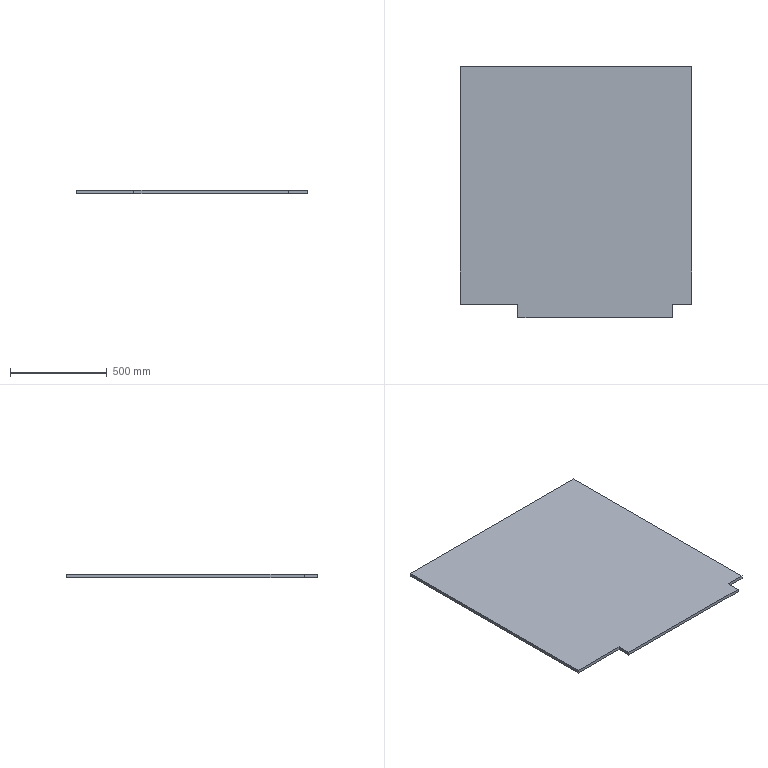Part | 1 solid | 10 faces | box 1198 x 1299 x 16 mm | volume 24453472 mm3 | plane 10
STEP:
#1=CARTESIAN_POINT('',(-599.,500.,0.));
#2=VERTEX_POINT('',#1);
#3=CARTESIAN_POINT('',(-599.,-729.,0.));
#4=VERTEX_POINT('',#3);
#5=CARTESIAN_POINT('',(-599.,500.,0.));
#6=DIRECTION('',(0.,-1.,0.));
#7=VECTOR('',#6,1000.);
#8=LINE('',#5,#7);
#9=EDGE_CURVE('',#2,#4,#8,.T.);
#10=ORIENTED_EDGE('',*,*,#9,.T.);
#11=CARTESIAN_POINT('',(-599.,-729.,16.));
#12=VERTEX_POINT('',#11);
#13=CARTESIAN_POINT('',(-599.,-729.,16.));
#14=DIRECTION('',(0.,0.,-1.));
#15=VECTOR('',#14,1000.);
#16=LINE('',#13,#15);
#17=EDGE_CURVE('',#12,#4,#16,.T.);
#18=ORIENTED_EDGE('',*,*,#17,.F.);
#19=CARTESIAN_POINT('',(-599.,500.,16.));
#20=VERTEX_POINT('',#19);
#21=CARTESIAN_POINT('',(-599.,500.,16.));
#22=DIRECTION('',(0.,-1.,0.));
#23=VECTOR('',#22,1000.);
#24=LINE('',#21,#23);
#25=EDGE_CURVE('',#20,#12,#24,.T.);
#26=ORIENTED_EDGE('',*,*,#25,.F.);
#27=CARTESIAN_POINT('',(-599.,500.,16.));
#28=DIRECTION('',(0.,0.,-1.));
#29=VECTOR('',#28,1000.);
#30=LINE('',#27,#29);
#31=EDGE_CURVE('',#20,#2,#30,.T.);
#32=ORIENTED_EDGE('',*,*,#31,.T.);
#33=EDGE_LOOP('',(#10,#18,#26,#32));
#34=FACE_OUTER_BOUND('',#33,.T.);
#35=CARTESIAN_POINT('',(-599.,500.,16.));
#36=DIRECTION('',(1.,0.,0.));
#37=DIRECTION('',(0.,1.,0.));
#38=AXIS2_PLACEMENT_3D('',#35,#36,#37);
#39=PLANE('',#38);
#40=ADVANCED_FACE('',(#34),#39,.F.);
#41=CARTESIAN_POINT('',(-300.,-729.,0.));
#42=VERTEX_POINT('',#41);
#43=CARTESIAN_POINT('',(-599.,-729.,0.));
#44=DIRECTION('',(1.,0.,0.));
#45=VECTOR('',#44,1000.);
#46=LINE('',#43,#45);
#47=EDGE_CURVE('',#4,#42,#46,.T.);
#48=ORIENTED_EDGE('',*,*,#47,.T.);
#49=CARTESIAN_POINT('',(-300.,-729.,16.));
#50=VERTEX_POINT('',#49);
#51=CARTESIAN_POINT('',(-300.,-729.,16.));
#52=DIRECTION('',(0.,0.,-1.));
#53=VECTOR('',#52,1000.);
#54=LINE('',#51,#53);
#55=EDGE_CURVE('',#50,#42,#54,.T.);
#56=ORIENTED_EDGE('',*,*,#55,.F.);
#57=CARTESIAN_POINT('',(-599.,-729.,16.));
#58=DIRECTION('',(1.,0.,0.));
#59=VECTOR('',#58,1000.);
#60=LINE('',#57,#59);
#61=EDGE_CURVE('',#12,#50,#60,.T.);
#62=ORIENTED_EDGE('',*,*,#61,.F.);
#63=ORIENTED_EDGE('',*,*,#17,.T.);
#64=EDGE_LOOP('',(#48,#56,#62,#63));
#65=FACE_OUTER_BOUND('',#64,.T.);
#66=CARTESIAN_POINT('',(-599.,-729.,16.));
#67=DIRECTION('',(0.,1.,0.));
#68=DIRECTION('',(0.,0.,1.));
#69=AXIS2_PLACEMENT_3D('',#66,#67,#68);
#70=PLANE('',#69);
#71=ADVANCED_FACE('',(#65),#70,.F.);
#72=CARTESIAN_POINT('',(-300.,-799.,0.));
#73=VERTEX_POINT('',#72);
#74=CARTESIAN_POINT('',(-300.,-729.,0.));
#75=DIRECTION('',(0.,-1.,0.));
#76=VECTOR('',#75,1000.);
#77=LINE('',#74,#76);
#78=EDGE_CURVE('',#42,#73,#77,.T.);
#79=ORIENTED_EDGE('',*,*,#78,.T.);
#80=CARTESIAN_POINT('',(-300.,-799.,16.));
#81=VERTEX_POINT('',#80);
#82=CARTESIAN_POINT('',(-300.,-799.,16.));
#83=DIRECTION('',(0.,0.,-1.));
#84=VECTOR('',#83,1000.);
#85=LINE('',#82,#84);
#86=EDGE_CURVE('',#81,#73,#85,.T.);
#87=ORIENTED_EDGE('',*,*,#86,.F.);
#88=CARTESIAN_POINT('',(-300.,-729.,16.));
#89=DIRECTION('',(0.,-1.,0.));
#90=VECTOR('',#89,1000.);
#91=LINE('',#88,#90);
#92=EDGE_CURVE('',#50,#81,#91,.T.);
#93=ORIENTED_EDGE('',*,*,#92,.F.);
#94=ORIENTED_EDGE('',*,*,#55,.T.);
#95=EDGE_LOOP('',(#79,#87,#93,#94));
#96=FACE_OUTER_BOUND('',#95,.T.);
#97=CARTESIAN_POINT('',(-300.,-729.,16.));
#98=DIRECTION('',(1.,0.,0.));
#99=DIRECTION('',(0.,0.,-1.));
#100=AXIS2_PLACEMENT_3D('',#97,#98,#99);
#101=PLANE('',#100);
#102=ADVANCED_FACE('',(#96),#101,.F.);
#103=CARTESIAN_POINT('',(500.,-799.,0.));
#104=VERTEX_POINT('',#103);
#105=CARTESIAN_POINT('',(-300.,-799.,0.));
#106=DIRECTION('',(1.,0.,0.));
#107=VECTOR('',#106,1000.);
#108=LINE('',#105,#107);
#109=EDGE_CURVE('',#73,#104,#108,.T.);
#110=ORIENTED_EDGE('',*,*,#109,.T.);
#111=CARTESIAN_POINT('',(500.,-799.,16.));
#112=VERTEX_POINT('',#111);
#113=CARTESIAN_POINT('',(500.,-799.,16.));
#114=DIRECTION('',(0.,0.,-1.));
#115=VECTOR('',#114,1000.);
#116=LINE('',#113,#115);
#117=EDGE_CURVE('',#112,#104,#116,.T.);
#118=ORIENTED_EDGE('',*,*,#117,.F.);
#119=CARTESIAN_POINT('',(-300.,-799.,16.));
#120=DIRECTION('',(1.,0.,0.));
#121=VECTOR('',#120,1000.);
#122=LINE('',#119,#121);
#123=EDGE_CURVE('',#81,#112,#122,.T.);
#124=ORIENTED_EDGE('',*,*,#123,.F.);
#125=ORIENTED_EDGE('',*,*,#86,.T.);
#126=EDGE_LOOP('',(#110,#118,#124,#125));
#127=FACE_OUTER_BOUND('',#126,.T.);
#128=CARTESIAN_POINT('',(-300.,-799.,16.));
#129=DIRECTION('',(0.,1.,0.));
#130=DIRECTION('',(0.,0.,1.));
#131=AXIS2_PLACEMENT_3D('',#128,#129,#130);
#132=PLANE('',#131);
#133=ADVANCED_FACE('',(#127),#132,.F.);
#134=CARTESIAN_POINT('',(500.,-729.,0.));
#135=VERTEX_POINT('',#134);
#136=CARTESIAN_POINT('',(500.,-799.,0.));
#137=DIRECTION('',(0.,1.,0.));
#138=VECTOR('',#137,1000.);
#139=LINE('',#136,#138);
#140=EDGE_CURVE('',#104,#135,#139,.T.);
#141=ORIENTED_EDGE('',*,*,#140,.T.);
#142=CARTESIAN_POINT('',(500.,-729.,16.));
#143=VERTEX_POINT('',#142);
#144=CARTESIAN_POINT('',(500.,-729.,16.));
#145=DIRECTION('',(0.,0.,-1.));
#146=VECTOR('',#145,1000.);
#147=LINE('',#144,#146);
#148=EDGE_CURVE('',#143,#135,#147,.T.);
#149=ORIENTED_EDGE('',*,*,#148,.F.);
#150=CARTESIAN_POINT('',(500.,-799.,16.));
#151=DIRECTION('',(0.,1.,0.));
#152=VECTOR('',#151,1000.);
#153=LINE('',#150,#152);
#154=EDGE_CURVE('',#112,#143,#153,.T.);
#155=ORIENTED_EDGE('',*,*,#154,.F.);
#156=ORIENTED_EDGE('',*,*,#117,.T.);
#157=EDGE_LOOP('',(#141,#149,#155,#156));
#158=FACE_OUTER_BOUND('',#157,.T.);
#159=CARTESIAN_POINT('',(500.,-799.,16.));
#160=DIRECTION('',(-1.,0.,0.));
#161=DIRECTION('',(0.,0.,1.));
#162=AXIS2_PLACEMENT_3D('',#159,#160,#161);
#163=PLANE('',#162);
#164=ADVANCED_FACE('',(#158),#163,.F.);
#165=CARTESIAN_POINT('',(599.,-729.,0.));
#166=VERTEX_POINT('',#165);
#167=CARTESIAN_POINT('',(500.,-729.,0.));
#168=DIRECTION('',(1.,0.,0.));
#169=VECTOR('',#168,1000.);
#170=LINE('',#167,#169);
#171=EDGE_CURVE('',#135,#166,#170,.T.);
#172=ORIENTED_EDGE('',*,*,#171,.T.);
#173=CARTESIAN_POINT('',(599.,-729.,16.));
#174=VERTEX_POINT('',#173);
#175=CARTESIAN_POINT('',(599.,-729.,16.));
#176=DIRECTION('',(0.,0.,-1.));
#177=VECTOR('',#176,1000.);
#178=LINE('',#175,#177);
#179=EDGE_CURVE('',#174,#166,#178,.T.);
#180=ORIENTED_EDGE('',*,*,#179,.F.);
#181=CARTESIAN_POINT('',(500.,-729.,16.));
#182=DIRECTION('',(1.,0.,0.));
#183=VECTOR('',#182,1000.);
#184=LINE('',#181,#183);
#185=EDGE_CURVE('',#143,#174,#184,.T.);
#186=ORIENTED_EDGE('',*,*,#185,.F.);
#187=ORIENTED_EDGE('',*,*,#148,.T.);
#188=EDGE_LOOP('',(#172,#180,#186,#187));
#189=FACE_OUTER_BOUND('',#188,.T.);
#190=CARTESIAN_POINT('',(500.,-729.,16.));
#191=DIRECTION('',(0.,1.,0.));
#192=DIRECTION('',(-1.,0.,0.));
#193=AXIS2_PLACEMENT_3D('',#190,#191,#192);
#194=PLANE('',#193);
#195=ADVANCED_FACE('',(#189),#194,.F.);
#196=CARTESIAN_POINT('',(599.,500.,0.));
#197=VERTEX_POINT('',#196);
#198=CARTESIAN_POINT('',(599.,500.,0.));
#199=DIRECTION('',(0.,1.,0.));
#200=VECTOR('',#199,1000.);
#201=LINE('',#198,#200);
#202=EDGE_CURVE('',#166,#197,#201,.T.);
#203=ORIENTED_EDGE('',*,*,#202,.T.);
#204=CARTESIAN_POINT('',(599.,500.,16.));
#205=VERTEX_POINT('',#204);
#206=CARTESIAN_POINT('',(599.,500.,16.));
#207=DIRECTION('',(0.,0.,-1.));
#208=VECTOR('',#207,1000.);
#209=LINE('',#206,#208);
#210=EDGE_CURVE('',#205,#197,#209,.T.);
#211=ORIENTED_EDGE('',*,*,#210,.F.);
#212=CARTESIAN_POINT('',(599.,500.,16.));
#213=DIRECTION('',(0.,1.,0.));
#214=VECTOR('',#213,1000.);
#215=LINE('',#212,#214);
#216=EDGE_CURVE('',#174,#205,#215,.T.);
#217=ORIENTED_EDGE('',*,*,#216,.F.);
#218=ORIENTED_EDGE('',*,*,#179,.T.);
#219=EDGE_LOOP('',(#203,#211,#217,#218));
#220=FACE_OUTER_BOUND('',#219,.T.);
#221=CARTESIAN_POINT('',(599.,500.,16.));
#222=DIRECTION('',(-1.,0.,0.));
#223=DIRECTION('',(0.,-1.,0.));
#224=AXIS2_PLACEMENT_3D('',#221,#222,#223);
#225=PLANE('',#224);
#226=ADVANCED_FACE('',(#220),#225,.F.);
#227=CARTESIAN_POINT('',(599.,500.,0.));
#228=DIRECTION('',(-1.,0.,0.));
#229=VECTOR('',#228,1000.);
#230=LINE('',#227,#229);
#231=EDGE_CURVE('',#197,#2,#230,.T.);
#232=ORIENTED_EDGE('',*,*,#231,.T.);
#233=ORIENTED_EDGE('',*,*,#31,.F.);
#234=CARTESIAN_POINT('',(599.,500.,16.));
#235=DIRECTION('',(-1.,0.,0.));
#236=VECTOR('',#235,1000.);
#237=LINE('',#234,#236);
#238=EDGE_CURVE('',#205,#20,#237,.T.);
#239=ORIENTED_EDGE('',*,*,#238,.F.);
#240=ORIENTED_EDGE('',*,*,#210,.T.);
#241=EDGE_LOOP('',(#232,#233,#239,#240));
#242=FACE_OUTER_BOUND('',#241,.T.);
#243=CARTESIAN_POINT('',(599.,500.,16.));
#244=DIRECTION('',(0.,-1.,0.));
#245=DIRECTION('',(1.,0.,0.));
#246=AXIS2_PLACEMENT_3D('',#243,#244,#245);
#247=PLANE('',#246);
#248=ADVANCED_FACE('',(#242),#247,.F.);
#249=ORIENTED_EDGE('',*,*,#25,.T.);
#250=ORIENTED_EDGE('',*,*,#61,.T.);
#251=ORIENTED_EDGE('',*,*,#92,.T.);
#252=ORIENTED_EDGE('',*,*,#123,.T.);
#253=ORIENTED_EDGE('',*,*,#154,.T.);
#254=ORIENTED_EDGE('',*,*,#185,.T.);
#255=ORIENTED_EDGE('',*,*,#216,.T.);
#256=ORIENTED_EDGE('',*,*,#238,.T.);
#257=EDGE_LOOP('',(#249,#250,#251,#252,#253,#254,#255,#256));
#258=FACE_OUTER_BOUND('',#257,.T.);
#259=CARTESIAN_POINT('',(0.,0.,16.));
#260=DIRECTION('',(0.,0.,1.));
#261=DIRECTION('',(1.,0.,0.));
#262=AXIS2_PLACEMENT_3D('',#259,#260,#261);
#263=PLANE('',#262);
#264=ADVANCED_FACE('',(#258),#263,.T.);
#265=ORIENTED_EDGE('',*,*,#9,.F.);
#266=ORIENTED_EDGE('',*,*,#231,.F.);
#267=ORIENTED_EDGE('',*,*,#202,.F.);
#268=ORIENTED_EDGE('',*,*,#171,.F.);
#269=ORIENTED_EDGE('',*,*,#140,.F.);
#270=ORIENTED_EDGE('',*,*,#109,.F.);
#271=ORIENTED_EDGE('',*,*,#78,.F.);
#272=ORIENTED_EDGE('',*,*,#47,.F.);
#273=EDGE_LOOP('',(#265,#266,#267,#268,#269,#270,#271,#272));
#274=FACE_OUTER_BOUND('',#273,.T.);
#275=CARTESIAN_POINT('',(0.,0.,0.));
#276=DIRECTION('',(0.,0.,1.));
#277=DIRECTION('',(1.,0.,0.));
#278=AXIS2_PLACEMENT_3D('',#275,#276,#277);
#279=PLANE('',#278);
#280=ADVANCED_FACE('',(#274),#279,.F.);
#281=CLOSED_SHELL('',(#40,#71,#102,#133,#164,#195,#226,#248,#264,#280));
#282=MANIFOLD_SOLID_BREP('',#281);
#283=CARTESIAN_POINT('',(0.,0.,0.));
#284=DIRECTION('',(0.,0.,1.));
#285=DIRECTION('',(1.,0.,0.));
#286=AXIS2_PLACEMENT_3D('',#283,#284,#285);
#287=(LENGTH_UNIT()NAMED_UNIT(*)SI_UNIT(.MILLI.,.METRE.));
#288=UNCERTAINTY_MEASURE_WITH_UNIT(LENGTH_MEASURE(0.00001),#287,'','');
#289=(NAMED_UNIT(*)PLANE_ANGLE_UNIT()SI_UNIT($,.RADIAN.));
#290=(NAMED_UNIT(*)SI_UNIT($,.STERADIAN.)SOLID_ANGLE_UNIT());
#291=(GEOMETRIC_REPRESENTATION_CONTEXT(3)GLOBAL_UNCERTAINTY_ASSIGNED_CONTEXT((#288))GLOBAL_UNIT_ASSIGNED_CONTEXT((#287,#289,#290))REPRESENTATION_CONTEXT('',''));
#292=ADVANCED_BREP_SHAPE_REPRESENTATION('',(#282,#286),#291);